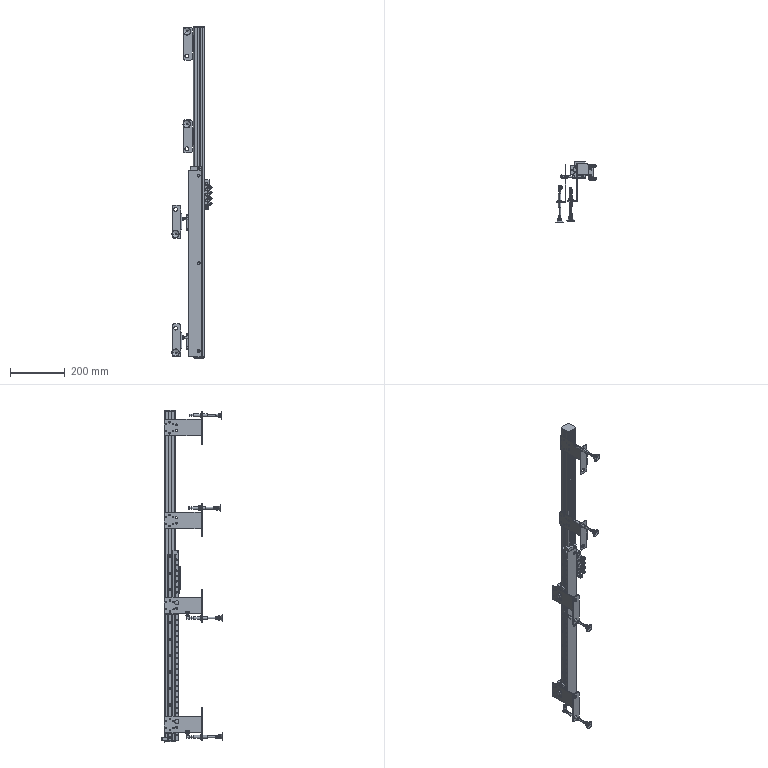Part | SolidWorks | features LocalLPattern 1, ReferencePattern 1 | 39 solids | 3071 faces | volume 1484218 mm3 | plane 1263 | cylinder 915 | cone 628 | spline 265 | commonest cylinder face diameters 4.1 x66 4 x56 7 x56 4.2 x48 10 x48 6 x44